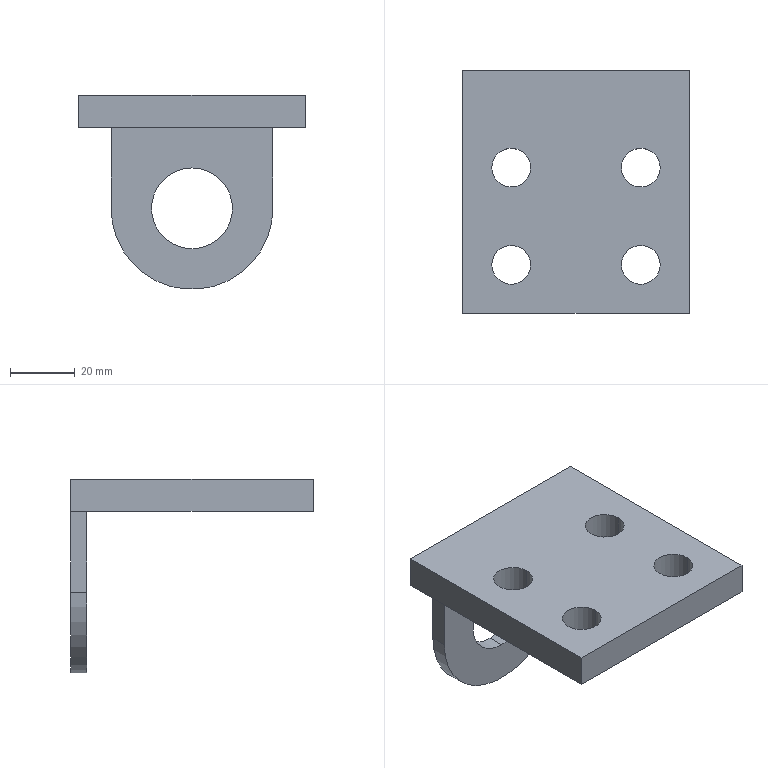Part | SolidWorks | features ICE 2, Extrusion 1 | 1 solid | 20 faces | box 70 x 75 x 60 mm | volume 56680 mm3 | cylinder 11 | plane 9 | commonest cylinder face diameters 12 x8 25 x2 50 x1
STEP:
#1=CARTESIAN_POINT('',(20.,55.,-12.5));
#2=VERTEX_POINT('',#1);
#3=CARTESIAN_POINT('',(20.,55.,-37.5));
#4=VERTEX_POINT('',#3);
#5=CARTESIAN_POINT('',(20.,55.,-25.));
#6=DIRECTION('',(0.,-1.,0.));
#7=DIRECTION('',(0.,0.,-1.));
#8=AXIS2_PLACEMENT_3D('',#5,#6,#7);
#9=CIRCLE('',#8,12.5);
#10=EDGE_CURVE('',#2,#4,#9,.T.);
#11=ORIENTED_EDGE('',*,*,#10,.T.);
#12=CARTESIAN_POINT('',(20.,60.,-37.5));
#13=VERTEX_POINT('',#12);
#14=CARTESIAN_POINT('',(20.,50.,-37.5));
#15=DIRECTION('',(0.,1.,0.));
#16=VECTOR('',#15,1000.);
#17=LINE('',#14,#16);
#18=EDGE_CURVE('',#4,#13,#17,.T.);
#19=ORIENTED_EDGE('',*,*,#18,.T.);
#20=CARTESIAN_POINT('',(20.,60.,-12.5));
#21=VERTEX_POINT('',#20);
#22=CARTESIAN_POINT('',(20.,60.,-25.));
#23=DIRECTION('',(0.,1.,0.));
#24=DIRECTION('',(0.,0.,1.));
#25=AXIS2_PLACEMENT_3D('',#22,#23,#24);
#26=CIRCLE('',#25,12.5);
#27=EDGE_CURVE('',#13,#21,#26,.T.);
#28=ORIENTED_EDGE('',*,*,#27,.T.);
#29=CARTESIAN_POINT('',(20.,50.,-12.5));
#30=DIRECTION('',(0.,1.,0.));
#31=VECTOR('',#30,1000.);
#32=LINE('',#29,#31);
#33=EDGE_CURVE('',#2,#21,#32,.T.);
#34=ORIENTED_EDGE('',*,*,#33,.F.);
#35=EDGE_LOOP('',(#11,#19,#28,#34));
#36=FACE_OUTER_BOUND('',#35,.T.);
#37=CARTESIAN_POINT('',(20.,50.,-25.));
#38=DIRECTION('',(0.,1.,0.));
#39=DIRECTION('',(0.,0.,1.));
#40=AXIS2_PLACEMENT_3D('',#37,#38,#39);
#41=CYLINDRICAL_SURFACE('',#40,12.5);
#42=ADVANCED_FACE('',(#36),#41,.F.);
#43=CARTESIAN_POINT('',(34.,0.,10.));
#44=VERTEX_POINT('',#43);
#45=CARTESIAN_POINT('',(46.,0.,10.));
#46=VERTEX_POINT('',#45);
#47=CARTESIAN_POINT('',(40.,0.,10.));
#48=DIRECTION('',(0.,0.,1.));
#49=DIRECTION('',(1.,0.,0.));
#50=AXIS2_PLACEMENT_3D('',#47,#48,#49);
#51=CIRCLE('',#50,6.);
#52=EDGE_CURVE('',#44,#46,#51,.T.);
#53=ORIENTED_EDGE('',*,*,#52,.T.);
#54=CARTESIAN_POINT('',(46.,0.,0.));
#55=VERTEX_POINT('',#54);
#56=CARTESIAN_POINT('',(46.,0.,10.));
#57=DIRECTION('',(0.,0.,-1.));
#58=VECTOR('',#57,1000.);
#59=LINE('',#56,#58);
#60=EDGE_CURVE('',#46,#55,#59,.T.);
#61=ORIENTED_EDGE('',*,*,#60,.T.);
#62=CARTESIAN_POINT('',(34.,0.,0.));
#63=VERTEX_POINT('',#62);
#64=CARTESIAN_POINT('',(40.,0.,0.));
#65=DIRECTION('',(0.,0.,1.));
#66=DIRECTION('',(1.,0.,0.));
#67=AXIS2_PLACEMENT_3D('',#64,#65,#66);
#68=CIRCLE('',#67,6.);
#69=EDGE_CURVE('',#63,#55,#68,.T.);
#70=ORIENTED_EDGE('',*,*,#69,.F.);
#71=CARTESIAN_POINT('',(34.,0.,10.));
#72=DIRECTION('',(0.,0.,-1.));
#73=VECTOR('',#72,1000.);
#74=LINE('',#71,#73);
#75=EDGE_CURVE('',#44,#63,#74,.T.);
#76=ORIENTED_EDGE('',*,*,#75,.F.);
#77=EDGE_LOOP('',(#53,#61,#70,#76));
#78=FACE_OUTER_BOUND('',#77,.T.);
#79=CARTESIAN_POINT('',(40.,0.,10.));
#80=DIRECTION('',(0.,0.,-1.));
#81=DIRECTION('',(-1.,0.,0.));
#82=AXIS2_PLACEMENT_3D('',#79,#80,#81);
#83=CYLINDRICAL_SURFACE('',#82,6.);
#84=ADVANCED_FACE('',(#78),#83,.F.);
#85=CARTESIAN_POINT('',(34.,30.,10.));
#86=VERTEX_POINT('',#85);
#87=CARTESIAN_POINT('',(46.,30.,10.));
#88=VERTEX_POINT('',#87);
#89=CARTESIAN_POINT('',(40.,30.,10.));
#90=DIRECTION('',(0.,0.,1.));
#91=DIRECTION('',(1.,0.,0.));
#92=AXIS2_PLACEMENT_3D('',#89,#90,#91);
#93=CIRCLE('',#92,6.);
#94=EDGE_CURVE('',#86,#88,#93,.T.);
#95=ORIENTED_EDGE('',*,*,#94,.T.);
#96=CARTESIAN_POINT('',(46.,30.,0.));
#97=VERTEX_POINT('',#96);
#98=CARTESIAN_POINT('',(46.,30.,10.));
#99=DIRECTION('',(0.,0.,-1.));
#100=VECTOR('',#99,1000.);
#101=LINE('',#98,#100);
#102=EDGE_CURVE('',#88,#97,#101,.T.);
#103=ORIENTED_EDGE('',*,*,#102,.T.);
#104=CARTESIAN_POINT('',(34.,30.,0.));
#105=VERTEX_POINT('',#104);
#106=CARTESIAN_POINT('',(40.,30.,0.));
#107=DIRECTION('',(0.,0.,1.));
#108=DIRECTION('',(1.,0.,0.));
#109=AXIS2_PLACEMENT_3D('',#106,#107,#108);
#110=CIRCLE('',#109,6.);
#111=EDGE_CURVE('',#105,#97,#110,.T.);
#112=ORIENTED_EDGE('',*,*,#111,.F.);
#113=CARTESIAN_POINT('',(34.,30.,10.));
#114=DIRECTION('',(0.,0.,-1.));
#115=VECTOR('',#114,1000.);
#116=LINE('',#113,#115);
#117=EDGE_CURVE('',#86,#105,#116,.T.);
#118=ORIENTED_EDGE('',*,*,#117,.F.);
#119=EDGE_LOOP('',(#95,#103,#112,#118));
#120=FACE_OUTER_BOUND('',#119,.T.);
#121=CARTESIAN_POINT('',(40.,30.,10.));
#122=DIRECTION('',(0.,0.,-1.));
#123=DIRECTION('',(-1.,0.,0.));
#124=AXIS2_PLACEMENT_3D('',#121,#122,#123);
#125=CYLINDRICAL_SURFACE('',#124,6.);
#126=ADVANCED_FACE('',(#120),#125,.F.);
#127=CARTESIAN_POINT('',(-6.,30.,10.));
#128=VERTEX_POINT('',#127);
#129=CARTESIAN_POINT('',(6.,30.,10.));
#130=VERTEX_POINT('',#129);
#131=CARTESIAN_POINT('',(0.,30.,10.));
#132=DIRECTION('',(0.,0.,1.));
#133=DIRECTION('',(1.,0.,0.));
#134=AXIS2_PLACEMENT_3D('',#131,#132,#133);
#135=CIRCLE('',#134,6.);
#136=EDGE_CURVE('',#128,#130,#135,.T.);
#137=ORIENTED_EDGE('',*,*,#136,.T.);
#138=CARTESIAN_POINT('',(6.,30.,0.));
#139=VERTEX_POINT('',#138);
#140=CARTESIAN_POINT('',(6.,30.,10.));
#141=DIRECTION('',(0.,0.,-1.));
#142=VECTOR('',#141,1000.);
#143=LINE('',#140,#142);
#144=EDGE_CURVE('',#130,#139,#143,.T.);
#145=ORIENTED_EDGE('',*,*,#144,.T.);
#146=CARTESIAN_POINT('',(-6.,30.,0.));
#147=VERTEX_POINT('',#146);
#148=CARTESIAN_POINT('',(0.,30.,0.));
#149=DIRECTION('',(0.,0.,1.));
#150=DIRECTION('',(1.,0.,0.));
#151=AXIS2_PLACEMENT_3D('',#148,#149,#150);
#152=CIRCLE('',#151,6.);
#153=EDGE_CURVE('',#147,#139,#152,.T.);
#154=ORIENTED_EDGE('',*,*,#153,.F.);
#155=CARTESIAN_POINT('',(-6.,30.,10.));
#156=DIRECTION('',(0.,0.,-1.));
#157=VECTOR('',#156,1000.);
#158=LINE('',#155,#157);
#159=EDGE_CURVE('',#128,#147,#158,.T.);
#160=ORIENTED_EDGE('',*,*,#159,.F.);
#161=EDGE_LOOP('',(#137,#145,#154,#160));
#162=FACE_OUTER_BOUND('',#161,.T.);
#163=CARTESIAN_POINT('',(0.,30.,10.));
#164=DIRECTION('',(0.,0.,-1.));
#165=DIRECTION('',(-1.,0.,0.));
#166=AXIS2_PLACEMENT_3D('',#163,#164,#165);
#167=CYLINDRICAL_SURFACE('',#166,6.);
#168=ADVANCED_FACE('',(#162),#167,.F.);
#169=CARTESIAN_POINT('',(-6.,0.,10.));
#170=VERTEX_POINT('',#169);
#171=CARTESIAN_POINT('',(6.,0.,10.));
#172=VERTEX_POINT('',#171);
#173=CARTESIAN_POINT('',(0.,0.,10.));
#174=DIRECTION('',(0.,0.,1.));
#175=DIRECTION('',(1.,0.,0.));
#176=AXIS2_PLACEMENT_3D('',#173,#174,#175);
#177=CIRCLE('',#176,6.);
#178=EDGE_CURVE('',#170,#172,#177,.T.);
#179=ORIENTED_EDGE('',*,*,#178,.T.);
#180=CARTESIAN_POINT('',(6.,0.,0.));
#181=VERTEX_POINT('',#180);
#182=CARTESIAN_POINT('',(6.,0.,10.));
#183=DIRECTION('',(0.,0.,-1.));
#184=VECTOR('',#183,1000.);
#185=LINE('',#182,#184);
#186=EDGE_CURVE('',#172,#181,#185,.T.);
#187=ORIENTED_EDGE('',*,*,#186,.T.);
#188=CARTESIAN_POINT('',(-6.,0.,0.));
#189=VERTEX_POINT('',#188);
#190=CARTESIAN_POINT('',(0.,0.,0.));
#191=DIRECTION('',(0.,0.,1.));
#192=DIRECTION('',(1.,0.,0.));
#193=AXIS2_PLACEMENT_3D('',#190,#191,#192);
#194=CIRCLE('',#193,6.);
#195=EDGE_CURVE('',#189,#181,#194,.T.);
#196=ORIENTED_EDGE('',*,*,#195,.F.);
#197=CARTESIAN_POINT('',(-6.,0.,10.));
#198=DIRECTION('',(0.,0.,-1.));
#199=VECTOR('',#198,1000.);
#200=LINE('',#197,#199);
#201=EDGE_CURVE('',#170,#189,#200,.T.);
#202=ORIENTED_EDGE('',*,*,#201,.F.);
#203=EDGE_LOOP('',(#179,#187,#196,#202));
#204=FACE_OUTER_BOUND('',#203,.T.);
#205=CARTESIAN_POINT('',(0.,0.,10.));
#206=DIRECTION('',(0.,0.,-1.));
#207=DIRECTION('',(-1.,0.,0.));
#208=AXIS2_PLACEMENT_3D('',#205,#206,#207);
#209=CYLINDRICAL_SURFACE('',#208,6.);
#210=ADVANCED_FACE('',(#204),#209,.F.);
#211=ORIENTED_EDGE('',*,*,#94,.F.);
#212=CARTESIAN_POINT('',(40.,30.,10.));
#213=DIRECTION('',(0.,0.,1.));
#214=DIRECTION('',(1.,0.,0.));
#215=AXIS2_PLACEMENT_3D('',#212,#213,#214);
#216=CIRCLE('',#215,6.);
#217=EDGE_CURVE('',#88,#86,#216,.T.);
#218=ORIENTED_EDGE('',*,*,#217,.F.);
#219=EDGE_LOOP('',(#211,#218));
#220=FACE_BOUND('',#219,.T.);
#221=ORIENTED_EDGE('',*,*,#178,.F.);
#222=CARTESIAN_POINT('',(0.,0.,10.));
#223=DIRECTION('',(0.,0.,1.));
#224=DIRECTION('',(1.,0.,0.));
#225=AXIS2_PLACEMENT_3D('',#222,#223,#224);
#226=CIRCLE('',#225,6.);
#227=EDGE_CURVE('',#172,#170,#226,.T.);
#228=ORIENTED_EDGE('',*,*,#227,.F.);
#229=EDGE_LOOP('',(#221,#228));
#230=FACE_BOUND('',#229,.T.);
#231=CARTESIAN_POINT('',(-15.,60.,10.));
#232=VERTEX_POINT('',#231);
#233=CARTESIAN_POINT('',(-15.,-15.,10.));
#234=VERTEX_POINT('',#233);
#235=CARTESIAN_POINT('',(-15.,55.,10.));
#236=DIRECTION('',(0.,-1.,0.));
#237=VECTOR('',#236,1000.);
#238=LINE('',#235,#237);
#239=EDGE_CURVE('',#232,#234,#238,.T.);
#240=ORIENTED_EDGE('',*,*,#239,.T.);
#241=CARTESIAN_POINT('',(55.,-15.,10.));
#242=VERTEX_POINT('',#241);
#243=CARTESIAN_POINT('',(-15.,-15.,10.));
#244=DIRECTION('',(1.,0.,0.));
#245=VECTOR('',#244,1000.);
#246=LINE('',#243,#245);
#247=EDGE_CURVE('',#234,#242,#246,.T.);
#248=ORIENTED_EDGE('',*,*,#247,.T.);
#249=CARTESIAN_POINT('',(55.,60.,10.));
#250=VERTEX_POINT('',#249);
#251=CARTESIAN_POINT('',(55.,55.,10.));
#252=DIRECTION('',(0.,1.,0.));
#253=VECTOR('',#252,1000.);
#254=LINE('',#251,#253);
#255=EDGE_CURVE('',#242,#250,#254,.T.);
#256=ORIENTED_EDGE('',*,*,#255,.T.);
#257=CARTESIAN_POINT('',(-15.,60.,10.));
#258=DIRECTION('',(-1.,0.,0.));
#259=VECTOR('',#258,1000.);
#260=LINE('',#257,#259);
#261=EDGE_CURVE('',#250,#232,#260,.T.);
#262=ORIENTED_EDGE('',*,*,#261,.T.);
#263=EDGE_LOOP('',(#240,#248,#256,#262));
#264=FACE_OUTER_BOUND('',#263,.T.);
#265=ORIENTED_EDGE('',*,*,#136,.F.);
#266=CARTESIAN_POINT('',(0.,30.,10.));
#267=DIRECTION('',(0.,0.,1.));
#268=DIRECTION('',(1.,0.,0.));
#269=AXIS2_PLACEMENT_3D('',#266,#267,#268);
#270=CIRCLE('',#269,6.);
#271=EDGE_CURVE('',#130,#128,#270,.T.);
#272=ORIENTED_EDGE('',*,*,#271,.F.);
#273=EDGE_LOOP('',(#265,#272));
#274=FACE_BOUND('',#273,.T.);
#275=ORIENTED_EDGE('',*,*,#52,.F.);
#276=CARTESIAN_POINT('',(40.,0.,10.));
#277=DIRECTION('',(0.,0.,1.));
#278=DIRECTION('',(1.,0.,0.));
#279=AXIS2_PLACEMENT_3D('',#276,#277,#278);
#280=CIRCLE('',#279,6.);
#281=EDGE_CURVE('',#46,#44,#280,.T.);
#282=ORIENTED_EDGE('',*,*,#281,.F.);
#283=EDGE_LOOP('',(#275,#282));
#284=FACE_BOUND('',#283,.T.);
#285=CARTESIAN_POINT('',(0.,0.,10.));
#286=DIRECTION('',(0.,0.,1.));
#287=DIRECTION('',(1.,0.,0.));
#288=AXIS2_PLACEMENT_3D('',#285,#286,#287);
#289=PLANE('',#288);
#290=ADVANCED_FACE('',(#220,#230,#264,#274,#284),#289,.T.);
#291=CARTESIAN_POINT('',(-5.,55.,0.));
#292=VERTEX_POINT('',#291);
#293=CARTESIAN_POINT('',(-5.,60.,0.));
#294=VERTEX_POINT('',#293);
#295=CARTESIAN_POINT('',(-5.,50.,0.));
#296=DIRECTION('',(0.,1.,0.));
#297=VECTOR('',#296,1000.);
#298=LINE('',#295,#297);
#299=EDGE_CURVE('',#292,#294,#298,.T.);
#300=ORIENTED_EDGE('',*,*,#299,.F.);
#301=CARTESIAN_POINT('',(45.,55.,0.));
#302=VERTEX_POINT('',#301);
#303=CARTESIAN_POINT('',(-15.,55.,0.));
#304=DIRECTION('',(-1.,0.,0.));
#305=VECTOR('',#304,1000.);
#306=LINE('',#303,#305);
#307=EDGE_CURVE('',#302,#292,#306,.T.);
#308=ORIENTED_EDGE('',*,*,#307,.F.);
#309=CARTESIAN_POINT('',(45.,60.,0.));
#310=VERTEX_POINT('',#309);
#311=CARTESIAN_POINT('',(45.,50.,0.));
#312=DIRECTION('',(0.,1.,0.));
#313=VECTOR('',#312,1000.);
#314=LINE('',#311,#313);
#315=EDGE_CURVE('',#302,#310,#314,.T.);
#316=ORIENTED_EDGE('',*,*,#315,.T.);
#317=CARTESIAN_POINT('',(55.,60.,0.));
#318=VERTEX_POINT('',#317);
#319=CARTESIAN_POINT('',(45.,60.,0.));
#320=DIRECTION('',(1.,0.,0.));
#321=VECTOR('',#320,1000.);
#322=LINE('',#319,#321);
#323=EDGE_CURVE('',#310,#318,#322,.T.);
#324=ORIENTED_EDGE('',*,*,#323,.T.);
#325=CARTESIAN_POINT('',(55.,-15.,0.));
#326=VERTEX_POINT('',#325);
#327=CARTESIAN_POINT('',(55.,55.,0.));
#328=DIRECTION('',(0.,1.,0.));
#329=VECTOR('',#328,1000.);
#330=LINE('',#327,#329);
#331=EDGE_CURVE('',#326,#318,#330,.T.);
#332=ORIENTED_EDGE('',*,*,#331,.F.);
#333=CARTESIAN_POINT('',(-15.,-15.,0.));
#334=VERTEX_POINT('',#333);
#335=CARTESIAN_POINT('',(-15.,-15.,0.));
#336=DIRECTION('',(1.,0.,0.));
#337=VECTOR('',#336,1000.);
#338=LINE('',#335,#337);
#339=EDGE_CURVE('',#334,#326,#338,.T.);
#340=ORIENTED_EDGE('',*,*,#339,.F.);
#341=CARTESIAN_POINT('',(-15.,60.,0.));
#342=VERTEX_POINT('',#341);
#343=CARTESIAN_POINT('',(-15.,55.,0.));
#344=DIRECTION('',(0.,-1.,0.));
#345=VECTOR('',#344,1000.);
#346=LINE('',#343,#345);
#347=EDGE_CURVE('',#342,#334,#346,.T.);
#348=ORIENTED_EDGE('',*,*,#347,.F.);
#349=CARTESIAN_POINT('',(-23.268,60.,0.));
#350=DIRECTION('',(1.,0.,0.));
#351=VECTOR('',#350,1000.);
#352=LINE('',#349,#351);
#353=EDGE_CURVE('',#342,#294,#352,.T.);
#354=ORIENTED_EDGE('',*,*,#353,.T.);
#355=EDGE_LOOP('',(#300,#308,#316,#324,#332,#340,#348,#354));
#356=FACE_OUTER_BOUND('',#355,.T.);
#357=ORIENTED_EDGE('',*,*,#111,.T.);
#358=CARTESIAN_POINT('',(40.,30.,0.));
#359=DIRECTION('',(0.,0.,1.));
#360=DIRECTION('',(1.,0.,0.));
#361=AXIS2_PLACEMENT_3D('',#358,#359,#360);
#362=CIRCLE('',#361,6.);
#363=EDGE_CURVE('',#97,#105,#362,.T.);
#364=ORIENTED_EDGE('',*,*,#363,.T.);
#365=EDGE_LOOP('',(#357,#364));
#366=FACE_BOUND('',#365,.T.);
#367=ORIENTED_EDGE('',*,*,#195,.T.);
#368=CARTESIAN_POINT('',(0.,0.,0.));
#369=DIRECTION('',(0.,0.,1.));
#370=DIRECTION('',(1.,0.,0.));
#371=AXIS2_PLACEMENT_3D('',#368,#369,#370);
#372=CIRCLE('',#371,6.);
#373=EDGE_CURVE('',#181,#189,#372,.T.);
#374=ORIENTED_EDGE('',*,*,#373,.T.);
#375=EDGE_LOOP('',(#367,#374));
#376=FACE_BOUND('',#375,.T.);
#377=ORIENTED_EDGE('',*,*,#153,.T.);
#378=CARTESIAN_POINT('',(0.,30.,0.));
#379=DIRECTION('',(0.,0.,1.));
#380=DIRECTION('',(1.,0.,0.));
#381=AXIS2_PLACEMENT_3D('',#378,#379,#380);
#382=CIRCLE('',#381,6.);
#383=EDGE_CURVE('',#139,#147,#382,.T.);
#384=ORIENTED_EDGE('',*,*,#383,.T.);
#385=EDGE_LOOP('',(#377,#384));
#386=FACE_BOUND('',#385,.T.);
#387=ORIENTED_EDGE('',*,*,#69,.T.);
#388=CARTESIAN_POINT('',(40.,0.,0.));
#389=DIRECTION('',(0.,0.,1.));
#390=DIRECTION('',(1.,0.,0.));
#391=AXIS2_PLACEMENT_3D('',#388,#389,#390);
#392=CIRCLE('',#391,6.);
#393=EDGE_CURVE('',#55,#63,#392,.T.);
#394=ORIENTED_EDGE('',*,*,#393,.T.);
#395=EDGE_LOOP('',(#387,#394));
#396=FACE_BOUND('',#395,.T.);
#397=CARTESIAN_POINT('',(0.,0.,0.));
#398=DIRECTION('',(0.,0.,1.));
#399=DIRECTION('',(1.,0.,0.));
#400=AXIS2_PLACEMENT_3D('',#397,#398,#399);
#401=PLANE('',#400);
#402=ADVANCED_FACE('',(#356,#366,#376,#386,#396),#401,.F.);
#403=CARTESIAN_POINT('',(-15.,60.,-50.));
#404=DIRECTION('',(0.,0.,1.));
#405=VECTOR('',#404,1000.);
#406=LINE('',#403,#405);
#407=EDGE_CURVE('',#342,#232,#406,.T.);
#408=ORIENTED_EDGE('',*,*,#407,.F.);
#409=ORIENTED_EDGE('',*,*,#347,.T.);
#410=CARTESIAN_POINT('',(-15.,-15.,10.));
#411=DIRECTION('',(0.,0.,-1.));
#412=VECTOR('',#411,1000.);
#413=LINE('',#410,#412);
#414=EDGE_CURVE('',#234,#334,#413,.T.);
#415=ORIENTED_EDGE('',*,*,#414,.F.);
#416=ORIENTED_EDGE('',*,*,#239,.F.);
#417=EDGE_LOOP('',(#408,#409,#415,#416));
#418=FACE_OUTER_BOUND('',#417,.T.);
#419=CARTESIAN_POINT('',(-15.,55.,10.));
#420=DIRECTION('',(1.,0.,0.));
#421=DIRECTION('',(0.,1.,0.));
#422=AXIS2_PLACEMENT_3D('',#419,#420,#421);
#423=PLANE('',#422);
#424=ADVANCED_FACE('',(#418),#423,.F.);
#425=ORIENTED_EDGE('',*,*,#339,.T.);
#426=CARTESIAN_POINT('',(55.,-15.,10.));
#427=DIRECTION('',(0.,0.,-1.));
#428=VECTOR('',#427,1000.);
#429=LINE('',#426,#428);
#430=EDGE_CURVE('',#242,#326,#429,.T.);
#431=ORIENTED_EDGE('',*,*,#430,.F.);
#432=ORIENTED_EDGE('',*,*,#247,.F.);
#433=ORIENTED_EDGE('',*,*,#414,.T.);
#434=EDGE_LOOP('',(#425,#431,#432,#433));
#435=FACE_OUTER_BOUND('',#434,.T.);
#436=CARTESIAN_POINT('',(-15.,-15.,10.));
#437=DIRECTION('',(0.,1.,0.));
#438=DIRECTION('',(0.,0.,1.));
#439=AXIS2_PLACEMENT_3D('',#436,#437,#438);
#440=PLANE('',#439);
#441=ADVANCED_FACE('',(#435),#440,.F.);
#442=ORIENTED_EDGE('',*,*,#331,.T.);
#443=CARTESIAN_POINT('',(55.,60.,-50.));
#444=DIRECTION('',(0.,0.,1.));
#445=VECTOR('',#444,1000.);
#446=LINE('',#443,#445);
#447=EDGE_CURVE('',#318,#250,#446,.T.);
#448=ORIENTED_EDGE('',*,*,#447,.T.);
#449=ORIENTED_EDGE('',*,*,#255,.F.);
#450=ORIENTED_EDGE('',*,*,#430,.T.);
#451=EDGE_LOOP('',(#442,#448,#449,#450));
#452=FACE_OUTER_BOUND('',#451,.T.);
#453=CARTESIAN_POINT('',(55.,55.,10.));
#454=DIRECTION('',(-1.,0.,0.));
#455=DIRECTION('',(0.,0.,1.));
#456=AXIS2_PLACEMENT_3D('',#453,#454,#455);
#457=PLANE('',#456);
#458=ADVANCED_FACE('',(#452),#457,.F.);
#459=ORIENTED_EDGE('',*,*,#186,.F.);
#460=ORIENTED_EDGE('',*,*,#227,.T.);
#461=ORIENTED_EDGE('',*,*,#201,.T.);
#462=ORIENTED_EDGE('',*,*,#373,.F.);
#463=EDGE_LOOP('',(#459,#460,#461,#462));
#464=FACE_OUTER_BOUND('',#463,.T.);
#465=CARTESIAN_POINT('',(0.,0.,10.));
#466=DIRECTION('',(0.,0.,-1.));
#467=DIRECTION('',(-1.,0.,0.));
#468=AXIS2_PLACEMENT_3D('',#465,#466,#467);
#469=CYLINDRICAL_SURFACE('',#468,6.);
#470=ADVANCED_FACE('',(#464),#469,.F.);
#471=ORIENTED_EDGE('',*,*,#144,.F.);
#472=ORIENTED_EDGE('',*,*,#271,.T.);
#473=ORIENTED_EDGE('',*,*,#159,.T.);
#474=ORIENTED_EDGE('',*,*,#383,.F.);
#475=EDGE_LOOP('',(#471,#472,#473,#474));
#476=FACE_OUTER_BOUND('',#475,.T.);
#477=CARTESIAN_POINT('',(0.,30.,10.));
#478=DIRECTION('',(0.,0.,-1.));
#479=DIRECTION('',(-1.,0.,0.));
#480=AXIS2_PLACEMENT_3D('',#477,#478,#479);
#481=CYLINDRICAL_SURFACE('',#480,6.);
#482=ADVANCED_FACE('',(#476),#481,.F.);
#483=ORIENTED_EDGE('',*,*,#102,.F.);
#484=ORIENTED_EDGE('',*,*,#217,.T.);
#485=ORIENTED_EDGE('',*,*,#117,.T.);
#486=ORIENTED_EDGE('',*,*,#363,.F.);
#487=EDGE_LOOP('',(#483,#484,#485,#486));
#488=FACE_OUTER_BOUND('',#487,.T.);
#489=CARTESIAN_POINT('',(40.,30.,10.));
#490=DIRECTION('',(0.,0.,-1.));
#491=DIRECTION('',(-1.,0.,0.));
#492=AXIS2_PLACEMENT_3D('',#489,#490,#491);
#493=CYLINDRICAL_SURFACE('',#492,6.);
#494=ADVANCED_FACE('',(#488),#493,.F.);
#495=ORIENTED_EDGE('',*,*,#60,.F.);
#496=ORIENTED_EDGE('',*,*,#281,.T.);
#497=ORIENTED_EDGE('',*,*,#75,.T.);
#498=ORIENTED_EDGE('',*,*,#393,.F.);
#499=EDGE_LOOP('',(#495,#496,#497,#498));
#500=FACE_OUTER_BOUND('',#499,.T.);
#501=CARTESIAN_POINT('',(40.,0.,10.));
#502=DIRECTION('',(0.,0.,-1.));
#503=DIRECTION('',(-1.,0.,0.));
#504=AXIS2_PLACEMENT_3D('',#501,#502,#503);
#505=CYLINDRICAL_SURFACE('',#504,6.);
#506=ADVANCED_FACE('',(#500),#505,.F.);
#507=ORIENTED_EDGE('',*,*,#353,.F.);
#508=ORIENTED_EDGE('',*,*,#407,.T.);
#509=ORIENTED_EDGE('',*,*,#261,.F.);
#510=ORIENTED_EDGE('',*,*,#447,.F.);
#511=ORIENTED_EDGE('',*,*,#323,.F.);
#512=CARTESIAN_POINT('',(45.,60.,-25.));
#513=VERTEX_POINT('',#512);
#514=CARTESIAN_POINT('',(45.,60.,-25.));
#515=DIRECTION('',(0.,0.,1.));
#516=VECTOR('',#515,1000.);
#517=LINE('',#514,#516);
#518=EDGE_CURVE('',#513,#310,#517,.T.);
#519=ORIENTED_EDGE('',*,*,#518,.F.);
#520=CARTESIAN_POINT('',(-5.,60.,-25.));
#521=VERTEX_POINT('',#520);
#522=CARTESIAN_POINT('',(20.,60.,-25.));
#523=DIRECTION('',(0.,-1.,0.));
#524=DIRECTION('',(0.,0.,1.));
#525=AXIS2_PLACEMENT_3D('',#522,#523,#524);
#526=CIRCLE('',#525,25.);
#527=EDGE_CURVE('',#521,#513,#526,.T.);
#528=ORIENTED_EDGE('',*,*,#527,.F.);
#529=CARTESIAN_POINT('',(-5.,60.,-25.));
#530=DIRECTION('',(0.,0.,-1.));
#531=VECTOR('',#530,1000.);
#532=LINE('',#529,#531);
#533=EDGE_CURVE('',#294,#521,#532,.T.);
#534=ORIENTED_EDGE('',*,*,#533,.F.);
#535=EDGE_LOOP('',(#507,#508,#509,#510,#511,#519,#528,#534));
#536=FACE_OUTER_BOUND('',#535,.T.);
#537=CARTESIAN_POINT('',(20.,60.,-25.));
#538=DIRECTION('',(0.,1.,0.));
#539=DIRECTION('',(0.,0.,1.));
#540=AXIS2_PLACEMENT_3D('',#537,#538,#539);
#541=CIRCLE('',#540,12.5);
#542=EDGE_CURVE('',#21,#13,#541,.T.);
#543=ORIENTED_EDGE('',*,*,#542,.F.);
#544=ORIENTED_EDGE('',*,*,#27,.F.);
#545=EDGE_LOOP('',(#543,#544));
#546=FACE_BOUND('',#545,.T.);
#547=CARTESIAN_POINT('',(-15.,60.,-50.));
#548=DIRECTION('',(0.,1.,0.));
#549=DIRECTION('',(0.,0.,1.));
#550=AXIS2_PLACEMENT_3D('',#547,#548,#549);
#551=PLANE('',#550);
#552=ADVANCED_FACE('',(#536,#546),#551,.T.);
#553=CARTESIAN_POINT('',(-5.,55.,-25.));
#554=VERTEX_POINT('',#553);
#555=CARTESIAN_POINT('',(-5.,55.,-50.));
#556=DIRECTION('',(0.,0.,1.));
#557=VECTOR('',#556,1000.);
#558=LINE('',#555,#557);
#559=EDGE_CURVE('',#554,#292,#558,.T.);
#560=ORIENTED_EDGE('',*,*,#559,.F.);
#561=CARTESIAN_POINT('',(45.,55.,-25.));
#562=VERTEX_POINT('',#561);
#563=CARTESIAN_POINT('',(20.,55.,-25.));
#564=DIRECTION('',(0.,1.,0.));
#565=DIRECTION('',(0.,0.,-1.));
#566=AXIS2_PLACEMENT_3D('',#563,#564,#565);
#567=CIRCLE('',#566,25.);
#568=EDGE_CURVE('',#562,#554,#567,.T.);
#569=ORIENTED_EDGE('',*,*,#568,.F.);
#570=CARTESIAN_POINT('',(45.,55.,-50.));
#571=DIRECTION('',(0.,0.,-1.));
#572=VECTOR('',#571,1000.);
#573=LINE('',#570,#572);
#574=EDGE_CURVE('',#302,#562,#573,.T.);
#575=ORIENTED_EDGE('',*,*,#574,.F.);
#576=ORIENTED_EDGE('',*,*,#307,.T.);
#577=EDGE_LOOP('',(#560,#569,#575,#576));
#578=FACE_OUTER_BOUND('',#577,.T.);
#579=ORIENTED_EDGE('',*,*,#10,.F.);
#580=CARTESIAN_POINT('',(20.,55.,-25.));
#581=DIRECTION('',(0.,-1.,0.));
#582=DIRECTION('',(0.,0.,-1.));
#583=AXIS2_PLACEMENT_3D('',#580,#581,#582);
#584=CIRCLE('',#583,12.5);
#585=EDGE_CURVE('',#4,#2,#584,.T.);
#586=ORIENTED_EDGE('',*,*,#585,.F.);
#587=EDGE_LOOP('',(#579,#586));
#588=FACE_BOUND('',#587,.T.);
#589=CARTESIAN_POINT('',(-15.,55.,-50.));
#590=DIRECTION('',(0.,-1.,0.));
#591=DIRECTION('',(0.,0.,-1.));
#592=AXIS2_PLACEMENT_3D('',#589,#590,#591);
#593=PLANE('',#592);
#594=ADVANCED_FACE('',(#578,#588),#593,.T.);
#595=ORIENTED_EDGE('',*,*,#18,.F.);
#596=ORIENTED_EDGE('',*,*,#585,.T.);
#597=ORIENTED_EDGE('',*,*,#33,.T.);
#598=ORIENTED_EDGE('',*,*,#542,.T.);
#599=EDGE_LOOP('',(#595,#596,#597,#598));
#600=FACE_OUTER_BOUND('',#599,.T.);
#601=CARTESIAN_POINT('',(20.,50.,-25.));
#602=DIRECTION('',(0.,1.,0.));
#603=DIRECTION('',(0.,0.,1.));
#604=AXIS2_PLACEMENT_3D('',#601,#602,#603);
#605=CYLINDRICAL_SURFACE('',#604,12.5);
#606=ADVANCED_FACE('',(#600),#605,.F.);
#607=ORIENTED_EDGE('',*,*,#568,.T.);
#608=CARTESIAN_POINT('',(-5.,50.,-25.));
#609=DIRECTION('',(0.,1.,0.));
#610=VECTOR('',#609,1000.);
#611=LINE('',#608,#610);
#612=EDGE_CURVE('',#554,#521,#611,.T.);
#613=ORIENTED_EDGE('',*,*,#612,.T.);
#614=ORIENTED_EDGE('',*,*,#527,.T.);
#615=CARTESIAN_POINT('',(45.,50.,-25.));
#616=DIRECTION('',(0.,1.,0.));
#617=VECTOR('',#616,1000.);
#618=LINE('',#615,#617);
#619=EDGE_CURVE('',#562,#513,#618,.T.);
#620=ORIENTED_EDGE('',*,*,#619,.F.);
#621=EDGE_LOOP('',(#607,#613,#614,#620));
#622=FACE_OUTER_BOUND('',#621,.T.);
#623=CARTESIAN_POINT('',(20.,50.,-25.));
#624=DIRECTION('',(0.,1.,0.));
#625=DIRECTION('',(0.,0.,1.));
#626=AXIS2_PLACEMENT_3D('',#623,#624,#625);
#627=CYLINDRICAL_SURFACE('',#626,25.);
#628=ADVANCED_FACE('',(#622),#627,.T.);
#629=ORIENTED_EDGE('',*,*,#559,.T.);
#630=ORIENTED_EDGE('',*,*,#299,.T.);
#631=ORIENTED_EDGE('',*,*,#533,.T.);
#632=ORIENTED_EDGE('',*,*,#612,.F.);
#633=EDGE_LOOP('',(#629,#630,#631,#632));
#634=FACE_OUTER_BOUND('',#633,.T.);
#635=CARTESIAN_POINT('',(-5.,50.,-25.));
#636=DIRECTION('',(1.,0.,0.));
#637=DIRECTION('',(0.,0.,-1.));
#638=AXIS2_PLACEMENT_3D('',#635,#636,#637);
#639=PLANE('',#638);
#640=ADVANCED_FACE('',(#634),#639,.F.);
#641=ORIENTED_EDGE('',*,*,#574,.T.);
#642=ORIENTED_EDGE('',*,*,#619,.T.);
#643=ORIENTED_EDGE('',*,*,#518,.T.);
#644=ORIENTED_EDGE('',*,*,#315,.F.);
#645=EDGE_LOOP('',(#641,#642,#643,#644));
#646=FACE_OUTER_BOUND('',#645,.T.);
#647=CARTESIAN_POINT('',(45.,50.,-25.));
#648=DIRECTION('',(-1.,0.,0.));
#649=DIRECTION('',(0.,0.,1.));
#650=AXIS2_PLACEMENT_3D('',#647,#648,#649);
#651=PLANE('',#650);
#652=ADVANCED_FACE('',(#646),#651,.F.);
#653=CLOSED_SHELL('',(#42,#84,#126,#168,#210,#290,#402,#424,#441,#458,#470,#482,#494,#506,#552,#594,#606,#628,#640,#652));
#654=MANIFOLD_SOLID_BREP('',#653);
#655=CARTESIAN_POINT('',(0.,0.,0.));
#656=DIRECTION('',(0.,0.,1.));
#657=DIRECTION('',(1.,0.,0.));
#658=AXIS2_PLACEMENT_3D('',#655,#656,#657);
#659=(LENGTH_UNIT()NAMED_UNIT(*)SI_UNIT(.MILLI.,.METRE.));
#660=UNCERTAINTY_MEASURE_WITH_UNIT(LENGTH_MEASURE(0.00001),#659,'','');
#661=(NAMED_UNIT(*)PLANE_ANGLE_UNIT()SI_UNIT($,.RADIAN.));
#662=(NAMED_UNIT(*)SI_UNIT($,.STERADIAN.)SOLID_ANGLE_UNIT());
#663=(GEOMETRIC_REPRESENTATION_CONTEXT(3)GLOBAL_UNCERTAINTY_ASSIGNED_CONTEXT((#660))GLOBAL_UNIT_ASSIGNED_CONTEXT((#659,#661,#662))REPRESENTATION_CONTEXT('',''));
#664=ADVANCED_BREP_SHAPE_REPRESENTATION('',(#654,#658),#663);